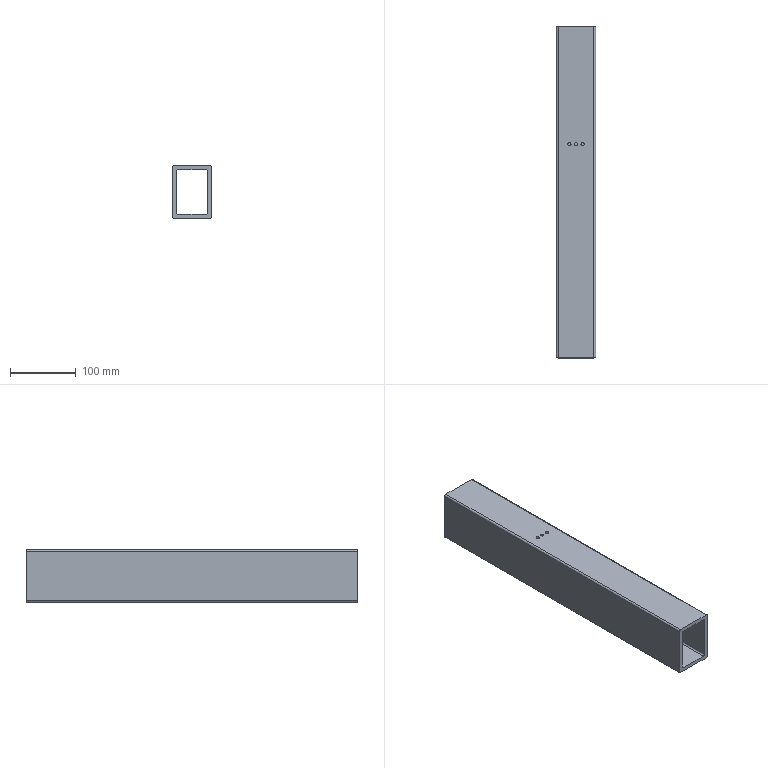Part | NX | 1 solid | 21 faces | box 60 x 505 x 80 mm | volume 775327 mm3 | cylinder 11 | plane 10 | commonest cylinder face diameters 5.236 x8 5 x3
STEP:
#1=CARTESIAN_POINT('',(746.,505.,37.382));
#2=VERTEX_POINT('',#1);
#3=CARTESIAN_POINT('',(746.,505.,-37.382));
#4=VERTEX_POINT('',#3);
#5=CARTESIAN_POINT('',(746.,505.,-37.382));
#6=DIRECTION('',(0.,0.,-1.));
#7=VECTOR('',#6,1000.);
#8=LINE('',#5,#7);
#9=EDGE_CURVE('',#2,#4,#8,.T.);
#10=ORIENTED_EDGE('',*,*,#9,.F.);
#11=CARTESIAN_POINT('',(746.,0.,37.382));
#12=VERTEX_POINT('',#11);
#13=CARTESIAN_POINT('',(746.,535.,37.382));
#14=DIRECTION('',(0.,-1.,0.));
#15=VECTOR('',#14,1000.);
#16=LINE('',#13,#15);
#17=EDGE_CURVE('',#2,#12,#16,.T.);
#18=ORIENTED_EDGE('',*,*,#17,.T.);
#19=CARTESIAN_POINT('',(746.,0.,-37.382));
#20=VERTEX_POINT('',#19);
#21=CARTESIAN_POINT('',(746.,0.,-37.382));
#22=DIRECTION('',(0.,0.,-1.));
#23=VECTOR('',#22,1000.);
#24=LINE('',#21,#23);
#25=EDGE_CURVE('',#12,#20,#24,.T.);
#26=ORIENTED_EDGE('',*,*,#25,.T.);
#27=CARTESIAN_POINT('',(746.,535.,-37.382));
#28=DIRECTION('',(0.,-1.,0.));
#29=VECTOR('',#28,1000.);
#30=LINE('',#27,#29);
#31=EDGE_CURVE('',#4,#20,#30,.T.);
#32=ORIENTED_EDGE('',*,*,#31,.F.);
#33=EDGE_LOOP('',(#10,#18,#26,#32));
#34=FACE_BOUND('',#33,.T.);
#35=CARTESIAN_POINT('',(746.,535.,-37.382));
#36=DIRECTION('',(-1.,0.,0.));
#37=DIRECTION('',(0.,0.,1.));
#38=AXIS2_PLACEMENT_3D('',#35,#36,#37);
#39=PLANE('',#38);
#40=ADVANCED_FACE('',(#34),#39,.F.);
#41=CARTESIAN_POINT('',(743.382,505.,40.));
#42=VERTEX_POINT('',#41);
#43=CARTESIAN_POINT('',(743.382,505.,37.382));
#44=DIRECTION('',(0.,1.,0.));
#45=DIRECTION('',(0.,0.,1.));
#46=AXIS2_PLACEMENT_3D('',#43,#44,#45);
#47=CIRCLE('',#46,2.618);
#48=EDGE_CURVE('',#42,#2,#47,.T.);
#49=ORIENTED_EDGE('',*,*,#48,.F.);
#50=CARTESIAN_POINT('',(743.382,0.,40.));
#51=VERTEX_POINT('',#50);
#52=CARTESIAN_POINT('',(743.382,535.,40.));
#53=DIRECTION('',(0.,-1.,0.));
#54=VECTOR('',#53,1000.);
#55=LINE('',#52,#54);
#56=EDGE_CURVE('',#42,#51,#55,.T.);
#57=ORIENTED_EDGE('',*,*,#56,.T.);
#58=CARTESIAN_POINT('',(743.382,0.,37.382));
#59=DIRECTION('',(0.,1.,0.));
#60=DIRECTION('',(0.,0.,1.));
#61=AXIS2_PLACEMENT_3D('',#58,#59,#60);
#62=CIRCLE('',#61,2.618);
#63=EDGE_CURVE('',#51,#12,#62,.T.);
#64=ORIENTED_EDGE('',*,*,#63,.T.);
#65=ORIENTED_EDGE('',*,*,#17,.F.);
#66=EDGE_LOOP('',(#49,#57,#64,#65));
#67=FACE_BOUND('',#66,.T.);
#68=CARTESIAN_POINT('',(743.382,535.,37.382));
#69=DIRECTION('',(0.,-1.,0.));
#70=DIRECTION('',(0.,0.,-1.));
#71=AXIS2_PLACEMENT_3D('',#68,#69,#70);
#72=CYLINDRICAL_SURFACE('',#71,2.618);
#73=ADVANCED_FACE('',(#67),#72,.T.);
#74=CARTESIAN_POINT('',(726.,322.5,40.));
#75=VERTEX_POINT('',#74);
#76=CARTESIAN_POINT('',(726.,325.,40.));
#77=DIRECTION('',(0.,0.,1.));
#78=DIRECTION('',(0.,-1.,0.));
#79=AXIS2_PLACEMENT_3D('',#76,#77,#78);
#80=CIRCLE('',#79,2.5);
#81=EDGE_CURVE('',#75,#75,#80,.T.);
#82=ORIENTED_EDGE('',*,*,#81,.F.);
#83=EDGE_LOOP('',(#82));
#84=FACE_BOUND('',#83,.T.);
#85=CARTESIAN_POINT('',(716.,322.5,40.));
#86=VERTEX_POINT('',#85);
#87=CARTESIAN_POINT('',(716.,325.,40.));
#88=DIRECTION('',(0.,0.,1.));
#89=DIRECTION('',(0.,-1.,0.));
#90=AXIS2_PLACEMENT_3D('',#87,#88,#89);
#91=CIRCLE('',#90,2.5);
#92=EDGE_CURVE('',#86,#86,#91,.T.);
#93=ORIENTED_EDGE('',*,*,#92,.F.);
#94=EDGE_LOOP('',(#93));
#95=FACE_BOUND('',#94,.T.);
#96=CARTESIAN_POINT('',(706.,322.5,40.));
#97=VERTEX_POINT('',#96);
#98=CARTESIAN_POINT('',(706.,325.,40.));
#99=DIRECTION('',(0.,0.,1.));
#100=DIRECTION('',(0.,-1.,0.));
#101=AXIS2_PLACEMENT_3D('',#98,#99,#100);
#102=CIRCLE('',#101,2.5);
#103=EDGE_CURVE('',#97,#97,#102,.T.);
#104=ORIENTED_EDGE('',*,*,#103,.F.);
#105=EDGE_LOOP('',(#104));
#106=FACE_BOUND('',#105,.T.);
#107=CARTESIAN_POINT('',(688.618,505.,40.));
#108=VERTEX_POINT('',#107);
#109=CARTESIAN_POINT('',(1126.,505.,40.));
#110=DIRECTION('',(-1.,0.,0.));
#111=VECTOR('',#110,1000.);
#112=LINE('',#109,#111);
#113=EDGE_CURVE('',#42,#108,#112,.T.);
#114=ORIENTED_EDGE('',*,*,#113,.T.);
#115=CARTESIAN_POINT('',(688.618,0.,40.));
#116=VERTEX_POINT('',#115);
#117=CARTESIAN_POINT('',(688.618,535.,40.));
#118=DIRECTION('',(0.,-1.,0.));
#119=VECTOR('',#118,1000.);
#120=LINE('',#117,#119);
#121=EDGE_CURVE('',#108,#116,#120,.T.);
#122=ORIENTED_EDGE('',*,*,#121,.T.);
#123=CARTESIAN_POINT('',(688.618,0.,40.));
#124=DIRECTION('',(1.,0.,0.));
#125=VECTOR('',#124,1000.);
#126=LINE('',#123,#125);
#127=EDGE_CURVE('',#116,#51,#126,.T.);
#128=ORIENTED_EDGE('',*,*,#127,.T.);
#129=ORIENTED_EDGE('',*,*,#56,.F.);
#130=EDGE_LOOP('',(#114,#122,#128,#129));
#131=FACE_BOUND('',#130,.T.);
#132=CARTESIAN_POINT('',(688.618,535.,40.));
#133=DIRECTION('',(0.,0.,-1.));
#134=DIRECTION('',(-1.,0.,0.));
#135=AXIS2_PLACEMENT_3D('',#132,#133,#134);
#136=PLANE('',#135);
#137=ADVANCED_FACE('',(#84,#95,#106,#131),#136,.F.);
#138=CARTESIAN_POINT('',(686.,505.,37.382));
#139=VERTEX_POINT('',#138);
#140=CARTESIAN_POINT('',(688.618,505.,37.382));
#141=DIRECTION('',(0.,1.,0.));
#142=DIRECTION('',(0.,0.,1.));
#143=AXIS2_PLACEMENT_3D('',#140,#141,#142);
#144=CIRCLE('',#143,2.618);
#145=EDGE_CURVE('',#139,#108,#144,.T.);
#146=ORIENTED_EDGE('',*,*,#145,.F.);
#147=CARTESIAN_POINT('',(686.,0.,37.382));
#148=VERTEX_POINT('',#147);
#149=CARTESIAN_POINT('',(686.,535.,37.382));
#150=DIRECTION('',(0.,-1.,0.));
#151=VECTOR('',#150,1000.);
#152=LINE('',#149,#151);
#153=EDGE_CURVE('',#139,#148,#152,.T.);
#154=ORIENTED_EDGE('',*,*,#153,.T.);
#155=CARTESIAN_POINT('',(688.618,0.,37.382));
#156=DIRECTION('',(0.,1.,0.));
#157=DIRECTION('',(0.,0.,1.));
#158=AXIS2_PLACEMENT_3D('',#155,#156,#157);
#159=CIRCLE('',#158,2.618);
#160=EDGE_CURVE('',#148,#116,#159,.T.);
#161=ORIENTED_EDGE('',*,*,#160,.T.);
#162=ORIENTED_EDGE('',*,*,#121,.F.);
#163=EDGE_LOOP('',(#146,#154,#161,#162));
#164=FACE_BOUND('',#163,.T.);
#165=CARTESIAN_POINT('',(688.618,535.,37.382));
#166=DIRECTION('',(0.,-1.,0.));
#167=DIRECTION('',(0.,0.,-1.));
#168=AXIS2_PLACEMENT_3D('',#165,#166,#167);
#169=CYLINDRICAL_SURFACE('',#168,2.618);
#170=ADVANCED_FACE('',(#164),#169,.T.);
#171=CARTESIAN_POINT('',(686.,505.,-37.382));
#172=VERTEX_POINT('',#171);
#173=CARTESIAN_POINT('',(686.,505.,-37.382));
#174=DIRECTION('',(0.,0.,1.));
#175=VECTOR('',#174,1000.);
#176=LINE('',#173,#175);
#177=EDGE_CURVE('',#172,#139,#176,.T.);
#178=ORIENTED_EDGE('',*,*,#177,.F.);
#179=CARTESIAN_POINT('',(686.,0.,-37.382));
#180=VERTEX_POINT('',#179);
#181=CARTESIAN_POINT('',(686.,535.,-37.382));
#182=DIRECTION('',(0.,-1.,0.));
#183=VECTOR('',#182,1000.);
#184=LINE('',#181,#183);
#185=EDGE_CURVE('',#172,#180,#184,.T.);
#186=ORIENTED_EDGE('',*,*,#185,.T.);
#187=CARTESIAN_POINT('',(686.,0.,-37.382));
#188=DIRECTION('',(0.,0.,1.));
#189=VECTOR('',#188,1000.);
#190=LINE('',#187,#189);
#191=EDGE_CURVE('',#180,#148,#190,.T.);
#192=ORIENTED_EDGE('',*,*,#191,.T.);
#193=ORIENTED_EDGE('',*,*,#153,.F.);
#194=EDGE_LOOP('',(#178,#186,#192,#193));
#195=FACE_BOUND('',#194,.T.);
#196=CARTESIAN_POINT('',(686.,535.,-37.382));
#197=DIRECTION('',(1.,0.,0.));
#198=DIRECTION('',(0.,0.,-1.));
#199=AXIS2_PLACEMENT_3D('',#196,#197,#198);
#200=PLANE('',#199);
#201=ADVANCED_FACE('',(#195),#200,.F.);
#202=CARTESIAN_POINT('',(688.618,505.,-40.));
#203=VERTEX_POINT('',#202);
#204=CARTESIAN_POINT('',(688.618,505.,-37.382));
#205=DIRECTION('',(0.,1.,0.));
#206=DIRECTION('',(0.,0.,1.));
#207=AXIS2_PLACEMENT_3D('',#204,#205,#206);
#208=CIRCLE('',#207,2.618);
#209=EDGE_CURVE('',#203,#172,#208,.T.);
#210=ORIENTED_EDGE('',*,*,#209,.F.);
#211=CARTESIAN_POINT('',(688.618,0.,-40.));
#212=VERTEX_POINT('',#211);
#213=CARTESIAN_POINT('',(688.618,535.,-40.));
#214=DIRECTION('',(0.,-1.,0.));
#215=VECTOR('',#214,1000.);
#216=LINE('',#213,#215);
#217=EDGE_CURVE('',#203,#212,#216,.T.);
#218=ORIENTED_EDGE('',*,*,#217,.T.);
#219=CARTESIAN_POINT('',(688.618,0.,-37.382));
#220=DIRECTION('',(0.,1.,0.));
#221=DIRECTION('',(0.,0.,1.));
#222=AXIS2_PLACEMENT_3D('',#219,#220,#221);
#223=CIRCLE('',#222,2.618);
#224=EDGE_CURVE('',#212,#180,#223,.T.);
#225=ORIENTED_EDGE('',*,*,#224,.T.);
#226=ORIENTED_EDGE('',*,*,#185,.F.);
#227=EDGE_LOOP('',(#210,#218,#225,#226));
#228=FACE_BOUND('',#227,.T.);
#229=CARTESIAN_POINT('',(688.618,535.,-37.382));
#230=DIRECTION('',(0.,-1.,0.));
#231=DIRECTION('',(0.,0.,-1.));
#232=AXIS2_PLACEMENT_3D('',#229,#230,#231);
#233=CYLINDRICAL_SURFACE('',#232,2.618);
#234=ADVANCED_FACE('',(#228),#233,.T.);
#235=CARTESIAN_POINT('',(743.382,505.,-40.));
#236=VERTEX_POINT('',#235);
#237=CARTESIAN_POINT('',(1126.,505.,-40.));
#238=DIRECTION('',(-1.,0.,0.));
#239=VECTOR('',#238,1000.);
#240=LINE('',#237,#239);
#241=EDGE_CURVE('',#236,#203,#240,.T.);
#242=ORIENTED_EDGE('',*,*,#241,.F.);
#243=CARTESIAN_POINT('',(743.382,0.,-40.));
#244=VERTEX_POINT('',#243);
#245=CARTESIAN_POINT('',(743.382,535.,-40.));
#246=DIRECTION('',(0.,-1.,0.));
#247=VECTOR('',#246,1000.);
#248=LINE('',#245,#247);
#249=EDGE_CURVE('',#236,#244,#248,.T.);
#250=ORIENTED_EDGE('',*,*,#249,.T.);
#251=CARTESIAN_POINT('',(688.618,0.,-40.));
#252=DIRECTION('',(-1.,0.,0.));
#253=VECTOR('',#252,1000.);
#254=LINE('',#251,#253);
#255=EDGE_CURVE('',#244,#212,#254,.T.);
#256=ORIENTED_EDGE('',*,*,#255,.T.);
#257=ORIENTED_EDGE('',*,*,#217,.F.);
#258=EDGE_LOOP('',(#242,#250,#256,#257));
#259=FACE_BOUND('',#258,.T.);
#260=CARTESIAN_POINT('',(688.618,535.,-40.));
#261=DIRECTION('',(0.,0.,1.));
#262=DIRECTION('',(1.,0.,0.));
#263=AXIS2_PLACEMENT_3D('',#260,#261,#262);
#264=PLANE('',#263);
#265=ADVANCED_FACE('',(#259),#264,.F.);
#266=CARTESIAN_POINT('',(743.382,505.,-37.382));
#267=DIRECTION('',(0.,1.,0.));
#268=DIRECTION('',(0.,0.,1.));
#269=AXIS2_PLACEMENT_3D('',#266,#267,#268);
#270=CIRCLE('',#269,2.618);
#271=EDGE_CURVE('',#4,#236,#270,.T.);
#272=ORIENTED_EDGE('',*,*,#271,.F.);
#273=ORIENTED_EDGE('',*,*,#31,.T.);
#274=CARTESIAN_POINT('',(743.382,0.,-37.382));
#275=DIRECTION('',(0.,1.,0.));
#276=DIRECTION('',(0.,0.,-1.));
#277=AXIS2_PLACEMENT_3D('',#274,#275,#276);
#278=CIRCLE('',#277,2.618);
#279=EDGE_CURVE('',#20,#244,#278,.T.);
#280=ORIENTED_EDGE('',*,*,#279,.T.);
#281=ORIENTED_EDGE('',*,*,#249,.F.);
#282=EDGE_LOOP('',(#272,#273,#280,#281));
#283=FACE_BOUND('',#282,.T.);
#284=CARTESIAN_POINT('',(743.382,535.,-37.382));
#285=DIRECTION('',(0.,-1.,0.));
#286=DIRECTION('',(0.,0.,-1.));
#287=AXIS2_PLACEMENT_3D('',#284,#285,#286);
#288=CYLINDRICAL_SURFACE('',#287,2.618);
#289=ADVANCED_FACE('',(#283),#288,.T.);
#290=ORIENTED_EDGE('',*,*,#279,.F.);
#291=ORIENTED_EDGE('',*,*,#25,.F.);
#292=ORIENTED_EDGE('',*,*,#63,.F.);
#293=ORIENTED_EDGE('',*,*,#127,.F.);
#294=ORIENTED_EDGE('',*,*,#160,.F.);
#295=ORIENTED_EDGE('',*,*,#191,.F.);
#296=ORIENTED_EDGE('',*,*,#224,.F.);
#297=ORIENTED_EDGE('',*,*,#255,.F.);
#298=EDGE_LOOP('',(#290,#291,#292,#293,#294,#295,#296,#297));
#299=FACE_BOUND('',#298,.T.);
#300=CARTESIAN_POINT('',(692.,0.,31.382));
#301=VERTEX_POINT('',#300);
#302=CARTESIAN_POINT('',(694.618,0.,34.));
#303=VERTEX_POINT('',#302);
#304=CARTESIAN_POINT('',(694.618,0.,31.382));
#305=DIRECTION('',(0.,1.,0.));
#306=DIRECTION('',(0.,0.,-1.));
#307=AXIS2_PLACEMENT_3D('',#304,#305,#306);
#308=CIRCLE('',#307,2.618);
#309=EDGE_CURVE('',#301,#303,#308,.T.);
#310=ORIENTED_EDGE('',*,*,#309,.T.);
#311=CARTESIAN_POINT('',(737.382,0.,34.));
#312=VERTEX_POINT('',#311);
#313=CARTESIAN_POINT('',(694.618,0.,34.));
#314=DIRECTION('',(1.,0.,0.));
#315=VECTOR('',#314,1000.);
#316=LINE('',#313,#315);
#317=EDGE_CURVE('',#303,#312,#316,.T.);
#318=ORIENTED_EDGE('',*,*,#317,.T.);
#319=CARTESIAN_POINT('',(740.,0.,31.382));
#320=VERTEX_POINT('',#319);
#321=CARTESIAN_POINT('',(737.382,0.,31.382));
#322=DIRECTION('',(0.,1.,0.));
#323=DIRECTION('',(0.,0.,-1.));
#324=AXIS2_PLACEMENT_3D('',#321,#322,#323);
#325=CIRCLE('',#324,2.618);
#326=EDGE_CURVE('',#312,#320,#325,.T.);
#327=ORIENTED_EDGE('',*,*,#326,.T.);
#328=CARTESIAN_POINT('',(740.,0.,-31.382));
#329=VERTEX_POINT('',#328);
#330=CARTESIAN_POINT('',(740.,0.,-31.382));
#331=DIRECTION('',(0.,0.,-1.));
#332=VECTOR('',#331,1000.);
#333=LINE('',#330,#332);
#334=EDGE_CURVE('',#320,#329,#333,.T.);
#335=ORIENTED_EDGE('',*,*,#334,.T.);
#336=CARTESIAN_POINT('',(737.382,0.,-34.));
#337=VERTEX_POINT('',#336);
#338=CARTESIAN_POINT('',(737.382,0.,-31.382));
#339=DIRECTION('',(0.,1.,0.));
#340=DIRECTION('',(0.,0.,-1.));
#341=AXIS2_PLACEMENT_3D('',#338,#339,#340);
#342=CIRCLE('',#341,2.618);
#343=EDGE_CURVE('',#329,#337,#342,.T.);
#344=ORIENTED_EDGE('',*,*,#343,.T.);
#345=CARTESIAN_POINT('',(694.618,0.,-34.));
#346=VERTEX_POINT('',#345);
#347=CARTESIAN_POINT('',(694.618,0.,-34.));
#348=DIRECTION('',(-1.,0.,0.));
#349=VECTOR('',#348,1000.);
#350=LINE('',#347,#349);
#351=EDGE_CURVE('',#337,#346,#350,.T.);
#352=ORIENTED_EDGE('',*,*,#351,.T.);
#353=CARTESIAN_POINT('',(692.,0.,-31.382));
#354=VERTEX_POINT('',#353);
#355=CARTESIAN_POINT('',(694.618,0.,-31.382));
#356=DIRECTION('',(0.,1.,0.));
#357=DIRECTION('',(0.,0.,1.));
#358=AXIS2_PLACEMENT_3D('',#355,#356,#357);
#359=CIRCLE('',#358,2.618);
#360=EDGE_CURVE('',#346,#354,#359,.T.);
#361=ORIENTED_EDGE('',*,*,#360,.T.);
#362=CARTESIAN_POINT('',(692.,0.,-31.382));
#363=DIRECTION('',(0.,0.,1.));
#364=VECTOR('',#363,1000.);
#365=LINE('',#362,#364);
#366=EDGE_CURVE('',#354,#301,#365,.T.);
#367=ORIENTED_EDGE('',*,*,#366,.T.);
#368=EDGE_LOOP('',(#310,#318,#327,#335,#344,#352,#361,#367));
#369=FACE_BOUND('',#368,.T.);
#370=CARTESIAN_POINT('',(743.382,0.,-37.382));
#371=DIRECTION('',(0.,-1.,0.));
#372=DIRECTION('',(0.,0.,-1.));
#373=AXIS2_PLACEMENT_3D('',#370,#371,#372);
#374=PLANE('',#373);
#375=ADVANCED_FACE('',(#299,#369),#374,.T.);
#376=CARTESIAN_POINT('',(723.5,325.,34.));
#377=VERTEX_POINT('',#376);
#378=CARTESIAN_POINT('',(726.,325.,34.));
#379=DIRECTION('',(0.,0.,-1.));
#380=DIRECTION('',(-1.,0.,0.));
#381=AXIS2_PLACEMENT_3D('',#378,#379,#380);
#382=CIRCLE('',#381,2.5);
#383=EDGE_CURVE('',#377,#377,#382,.T.);
#384=ORIENTED_EDGE('',*,*,#383,.F.);
#385=EDGE_LOOP('',(#384));
#386=FACE_BOUND('',#385,.T.);
#387=CARTESIAN_POINT('',(713.5,325.,34.));
#388=VERTEX_POINT('',#387);
#389=CARTESIAN_POINT('',(716.,325.,34.));
#390=DIRECTION('',(0.,0.,-1.));
#391=DIRECTION('',(-1.,0.,0.));
#392=AXIS2_PLACEMENT_3D('',#389,#390,#391);
#393=CIRCLE('',#392,2.5);
#394=EDGE_CURVE('',#388,#388,#393,.T.);
#395=ORIENTED_EDGE('',*,*,#394,.F.);
#396=EDGE_LOOP('',(#395));
#397=FACE_BOUND('',#396,.T.);
#398=CARTESIAN_POINT('',(703.5,325.,34.));
#399=VERTEX_POINT('',#398);
#400=CARTESIAN_POINT('',(706.,325.,34.));
#401=DIRECTION('',(0.,0.,-1.));
#402=DIRECTION('',(-1.,0.,0.));
#403=AXIS2_PLACEMENT_3D('',#400,#401,#402);
#404=CIRCLE('',#403,2.5);
#405=EDGE_CURVE('',#399,#399,#404,.T.);
#406=ORIENTED_EDGE('',*,*,#405,.F.);
#407=EDGE_LOOP('',(#406));
#408=FACE_BOUND('',#407,.T.);
#409=CARTESIAN_POINT('',(694.618,505.,34.));
#410=VERTEX_POINT('',#409);
#411=CARTESIAN_POINT('',(694.618,535.,34.));
#412=DIRECTION('',(0.,-1.,0.));
#413=VECTOR('',#412,1000.);
#414=LINE('',#411,#413);
#415=EDGE_CURVE('',#410,#303,#414,.T.);
#416=ORIENTED_EDGE('',*,*,#415,.F.);
#417=CARTESIAN_POINT('',(737.382,505.,34.));
#418=VERTEX_POINT('',#417);
#419=CARTESIAN_POINT('',(694.618,505.,34.));
#420=DIRECTION('',(1.,0.,0.));
#421=VECTOR('',#420,1000.);
#422=LINE('',#419,#421);
#423=EDGE_CURVE('',#410,#418,#422,.T.);
#424=ORIENTED_EDGE('',*,*,#423,.T.);
#425=CARTESIAN_POINT('',(737.382,535.,34.));
#426=DIRECTION('',(0.,-1.,0.));
#427=VECTOR('',#426,1000.);
#428=LINE('',#425,#427);
#429=EDGE_CURVE('',#418,#312,#428,.T.);
#430=ORIENTED_EDGE('',*,*,#429,.T.);
#431=ORIENTED_EDGE('',*,*,#317,.F.);
#432=EDGE_LOOP('',(#416,#424,#430,#431));
#433=FACE_BOUND('',#432,.T.);
#434=CARTESIAN_POINT('',(694.618,535.,34.));
#435=DIRECTION('',(0.,0.,-1.));
#436=DIRECTION('',(-1.,0.,0.));
#437=AXIS2_PLACEMENT_3D('',#434,#435,#436);
#438=PLANE('',#437);
#439=ADVANCED_FACE('',(#386,#397,#408,#433),#438,.T.);
#440=ORIENTED_EDGE('',*,*,#429,.F.);
#441=CARTESIAN_POINT('',(740.,505.,31.382));
#442=VERTEX_POINT('',#441);
#443=CARTESIAN_POINT('',(737.382,505.,31.382));
#444=DIRECTION('',(0.,1.,0.));
#445=DIRECTION('',(0.,0.,1.));
#446=AXIS2_PLACEMENT_3D('',#443,#444,#445);
#447=CIRCLE('',#446,2.618);
#448=EDGE_CURVE('',#418,#442,#447,.T.);
#449=ORIENTED_EDGE('',*,*,#448,.T.);
#450=CARTESIAN_POINT('',(740.,535.,31.382));
#451=DIRECTION('',(0.,-1.,0.));
#452=VECTOR('',#451,1000.);
#453=LINE('',#450,#452);
#454=EDGE_CURVE('',#442,#320,#453,.T.);
#455=ORIENTED_EDGE('',*,*,#454,.T.);
#456=ORIENTED_EDGE('',*,*,#326,.F.);
#457=EDGE_LOOP('',(#440,#449,#455,#456));
#458=FACE_BOUND('',#457,.T.);
#459=CARTESIAN_POINT('',(737.382,535.,31.382));
#460=DIRECTION('',(0.,-1.,0.));
#461=DIRECTION('',(0.,0.,-1.));
#462=AXIS2_PLACEMENT_3D('',#459,#460,#461);
#463=CYLINDRICAL_SURFACE('',#462,2.618);
#464=ADVANCED_FACE('',(#458),#463,.F.);
#465=ORIENTED_EDGE('',*,*,#454,.F.);
#466=CARTESIAN_POINT('',(740.,505.,-31.382));
#467=VERTEX_POINT('',#466);
#468=CARTESIAN_POINT('',(740.,505.,-31.382));
#469=DIRECTION('',(0.,0.,-1.));
#470=VECTOR('',#469,1000.);
#471=LINE('',#468,#470);
#472=EDGE_CURVE('',#442,#467,#471,.T.);
#473=ORIENTED_EDGE('',*,*,#472,.T.);
#474=CARTESIAN_POINT('',(740.,535.,-31.382));
#475=DIRECTION('',(0.,-1.,0.));
#476=VECTOR('',#475,1000.);
#477=LINE('',#474,#476);
#478=EDGE_CURVE('',#467,#329,#477,.T.);
#479=ORIENTED_EDGE('',*,*,#478,.T.);
#480=ORIENTED_EDGE('',*,*,#334,.F.);
#481=EDGE_LOOP('',(#465,#473,#479,#480));
#482=FACE_BOUND('',#481,.T.);
#483=CARTESIAN_POINT('',(740.,535.,-31.382));
#484=DIRECTION('',(-1.,0.,0.));
#485=DIRECTION('',(0.,0.,1.));
#486=AXIS2_PLACEMENT_3D('',#483,#484,#485);
#487=PLANE('',#486);
#488=ADVANCED_FACE('',(#482),#487,.T.);
#489=ORIENTED_EDGE('',*,*,#478,.F.);
#490=CARTESIAN_POINT('',(737.382,505.,-34.));
#491=VERTEX_POINT('',#490);
#492=CARTESIAN_POINT('',(737.382,505.,-31.382));
#493=DIRECTION('',(0.,1.,0.));
#494=DIRECTION('',(0.,0.,1.));
#495=AXIS2_PLACEMENT_3D('',#492,#493,#494);
#496=CIRCLE('',#495,2.618);
#497=EDGE_CURVE('',#467,#491,#496,.T.);
#498=ORIENTED_EDGE('',*,*,#497,.T.);
#499=CARTESIAN_POINT('',(737.382,535.,-34.));
#500=DIRECTION('',(0.,-1.,0.));
#501=VECTOR('',#500,1000.);
#502=LINE('',#499,#501);
#503=EDGE_CURVE('',#491,#337,#502,.T.);
#504=ORIENTED_EDGE('',*,*,#503,.T.);
#505=ORIENTED_EDGE('',*,*,#343,.F.);
#506=EDGE_LOOP('',(#489,#498,#504,#505));
#507=FACE_BOUND('',#506,.T.);
#508=CARTESIAN_POINT('',(737.382,535.,-31.382));
#509=DIRECTION('',(0.,-1.,0.));
#510=DIRECTION('',(0.,0.,-1.));
#511=AXIS2_PLACEMENT_3D('',#508,#509,#510);
#512=CYLINDRICAL_SURFACE('',#511,2.618);
#513=ADVANCED_FACE('',(#507),#512,.F.);
#514=ORIENTED_EDGE('',*,*,#503,.F.);
#515=CARTESIAN_POINT('',(694.618,505.,-34.));
#516=VERTEX_POINT('',#515);
#517=CARTESIAN_POINT('',(694.618,505.,-34.));
#518=DIRECTION('',(-1.,0.,0.));
#519=VECTOR('',#518,1000.);
#520=LINE('',#517,#519);
#521=EDGE_CURVE('',#491,#516,#520,.T.);
#522=ORIENTED_EDGE('',*,*,#521,.T.);
#523=CARTESIAN_POINT('',(694.618,535.,-34.));
#524=DIRECTION('',(0.,-1.,0.));
#525=VECTOR('',#524,1000.);
#526=LINE('',#523,#525);
#527=EDGE_CURVE('',#516,#346,#526,.T.);
#528=ORIENTED_EDGE('',*,*,#527,.T.);
#529=ORIENTED_EDGE('',*,*,#351,.F.);
#530=EDGE_LOOP('',(#514,#522,#528,#529));
#531=FACE_BOUND('',#530,.T.);
#532=CARTESIAN_POINT('',(694.618,535.,-34.));
#533=DIRECTION('',(0.,0.,1.));
#534=DIRECTION('',(1.,0.,0.));
#535=AXIS2_PLACEMENT_3D('',#532,#533,#534);
#536=PLANE('',#535);
#537=ADVANCED_FACE('',(#531),#536,.T.);
#538=ORIENTED_EDGE('',*,*,#527,.F.);
#539=CARTESIAN_POINT('',(692.,505.,-31.382));
#540=VERTEX_POINT('',#539);
#541=CARTESIAN_POINT('',(694.618,505.,-31.382));
#542=DIRECTION('',(0.,1.,0.));
#543=DIRECTION('',(0.,0.,1.));
#544=AXIS2_PLACEMENT_3D('',#541,#542,#543);
#545=CIRCLE('',#544,2.618);
#546=EDGE_CURVE('',#516,#540,#545,.T.);
#547=ORIENTED_EDGE('',*,*,#546,.T.);
#548=CARTESIAN_POINT('',(692.,535.,-31.382));
#549=DIRECTION('',(0.,-1.,0.));
#550=VECTOR('',#549,1000.);
#551=LINE('',#548,#550);
#552=EDGE_CURVE('',#540,#354,#551,.T.);
#553=ORIENTED_EDGE('',*,*,#552,.T.);
#554=ORIENTED_EDGE('',*,*,#360,.F.);
#555=EDGE_LOOP('',(#538,#547,#553,#554));
#556=FACE_BOUND('',#555,.T.);
#557=CARTESIAN_POINT('',(694.618,535.,-31.382));
#558=DIRECTION('',(0.,-1.,0.));
#559=DIRECTION('',(0.,0.,-1.));
#560=AXIS2_PLACEMENT_3D('',#557,#558,#559);
#561=CYLINDRICAL_SURFACE('',#560,2.618);
#562=ADVANCED_FACE('',(#556),#561,.F.);
#563=ORIENTED_EDGE('',*,*,#552,.F.);
#564=CARTESIAN_POINT('',(692.,505.,31.382));
#565=VERTEX_POINT('',#564);
#566=CARTESIAN_POINT('',(692.,505.,-31.382));
#567=DIRECTION('',(0.,0.,1.));
#568=VECTOR('',#567,1000.);
#569=LINE('',#566,#568);
#570=EDGE_CURVE('',#540,#565,#569,.T.);
#571=ORIENTED_EDGE('',*,*,#570,.T.);
#572=CARTESIAN_POINT('',(692.,535.,31.382));
#573=DIRECTION('',(0.,-1.,0.));
#574=VECTOR('',#573,1000.);
#575=LINE('',#572,#574);
#576=EDGE_CURVE('',#565,#301,#575,.T.);
#577=ORIENTED_EDGE('',*,*,#576,.T.);
#578=ORIENTED_EDGE('',*,*,#366,.F.);
#579=EDGE_LOOP('',(#563,#571,#577,#578));
#580=FACE_BOUND('',#579,.T.);
#581=CARTESIAN_POINT('',(692.,535.,-31.382));
#582=DIRECTION('',(1.,0.,0.));
#583=DIRECTION('',(0.,0.,-1.));
#584=AXIS2_PLACEMENT_3D('',#581,#582,#583);
#585=PLANE('',#584);
#586=ADVANCED_FACE('',(#580),#585,.T.);
#587=ORIENTED_EDGE('',*,*,#576,.F.);
#588=CARTESIAN_POINT('',(694.618,505.,31.382));
#589=DIRECTION('',(0.,1.,0.));
#590=DIRECTION('',(0.,0.,1.));
#591=AXIS2_PLACEMENT_3D('',#588,#589,#590);
#592=CIRCLE('',#591,2.618);
#593=EDGE_CURVE('',#565,#410,#592,.T.);
#594=ORIENTED_EDGE('',*,*,#593,.T.);
#595=ORIENTED_EDGE('',*,*,#415,.T.);
#596=ORIENTED_EDGE('',*,*,#309,.F.);
#597=EDGE_LOOP('',(#587,#594,#595,#596));
#598=FACE_BOUND('',#597,.T.);
#599=CARTESIAN_POINT('',(694.618,535.,31.382));
#600=DIRECTION('',(0.,-1.,0.));
#601=DIRECTION('',(0.,0.,-1.));
#602=AXIS2_PLACEMENT_3D('',#599,#600,#601);
#603=CYLINDRICAL_SURFACE('',#602,2.618);
#604=ADVANCED_FACE('',(#598),#603,.F.);
#605=ORIENTED_EDGE('',*,*,#570,.F.);
#606=ORIENTED_EDGE('',*,*,#546,.F.);
#607=ORIENTED_EDGE('',*,*,#521,.F.);
#608=ORIENTED_EDGE('',*,*,#497,.F.);
#609=ORIENTED_EDGE('',*,*,#472,.F.);
#610=ORIENTED_EDGE('',*,*,#448,.F.);
#611=ORIENTED_EDGE('',*,*,#423,.F.);
#612=ORIENTED_EDGE('',*,*,#593,.F.);
#613=EDGE_LOOP('',(#605,#606,#607,#608,#609,#610,#611,#612));
#614=FACE_BOUND('',#613,.T.);
#615=ORIENTED_EDGE('',*,*,#209,.T.);
#616=ORIENTED_EDGE('',*,*,#177,.T.);
#617=ORIENTED_EDGE('',*,*,#145,.T.);
#618=ORIENTED_EDGE('',*,*,#113,.F.);
#619=ORIENTED_EDGE('',*,*,#48,.T.);
#620=ORIENTED_EDGE('',*,*,#9,.T.);
#621=ORIENTED_EDGE('',*,*,#271,.T.);
#622=ORIENTED_EDGE('',*,*,#241,.T.);
#623=EDGE_LOOP('',(#615,#616,#617,#618,#619,#620,#621,#622));
#624=FACE_BOUND('',#623,.T.);
#625=CARTESIAN_POINT('',(1126.,505.,37.382));
#626=DIRECTION('',(0.,1.,0.));
#627=DIRECTION('',(0.,0.,1.));
#628=AXIS2_PLACEMENT_3D('',#625,#626,#627);
#629=PLANE('',#628);
#630=ADVANCED_FACE('',(#614,#624),#629,.T.);
#631=ORIENTED_EDGE('',*,*,#405,.T.);
#632=EDGE_LOOP('',(#631));
#633=FACE_BOUND('',#632,.T.);
#634=ORIENTED_EDGE('',*,*,#103,.T.);
#635=EDGE_LOOP('',(#634));
#636=FACE_BOUND('',#635,.T.);
#637=CARTESIAN_POINT('',(706.,325.,40.));
#638=DIRECTION('',(0.,0.,1.));
#639=DIRECTION('',(0.,-1.,0.));
#640=AXIS2_PLACEMENT_3D('',#637,#638,#639);
#641=CYLINDRICAL_SURFACE('',#640,2.5);
#642=ADVANCED_FACE('',(#633,#636),#641,.F.);
#643=ORIENTED_EDGE('',*,*,#394,.T.);
#644=EDGE_LOOP('',(#643));
#645=FACE_BOUND('',#644,.T.);
#646=ORIENTED_EDGE('',*,*,#92,.T.);
#647=EDGE_LOOP('',(#646));
#648=FACE_BOUND('',#647,.T.);
#649=CARTESIAN_POINT('',(716.,325.,40.));
#650=DIRECTION('',(0.,0.,1.));
#651=DIRECTION('',(0.,-1.,0.));
#652=AXIS2_PLACEMENT_3D('',#649,#650,#651);
#653=CYLINDRICAL_SURFACE('',#652,2.5);
#654=ADVANCED_FACE('',(#645,#648),#653,.F.);
#655=ORIENTED_EDGE('',*,*,#383,.T.);
#656=EDGE_LOOP('',(#655));
#657=FACE_BOUND('',#656,.T.);
#658=ORIENTED_EDGE('',*,*,#81,.T.);
#659=EDGE_LOOP('',(#658));
#660=FACE_BOUND('',#659,.T.);
#661=CARTESIAN_POINT('',(726.,325.,40.));
#662=DIRECTION('',(0.,0.,1.));
#663=DIRECTION('',(0.,-1.,0.));
#664=AXIS2_PLACEMENT_3D('',#661,#662,#663);
#665=CYLINDRICAL_SURFACE('',#664,2.5);
#666=ADVANCED_FACE('',(#657,#660),#665,.F.);
#667=CLOSED_SHELL('',(#40,#73,#137,#170,#201,#234,#265,#289,#375,#439,#464,#488,#513,#537,#562,#586,#604,#630,#642,#654,#666));
#668=MANIFOLD_SOLID_BREP('',#667);
#669=(LENGTH_UNIT()NAMED_UNIT(*)SI_UNIT(.MILLI.,.METRE.));
#670=UNCERTAINTY_MEASURE_WITH_UNIT(LENGTH_MEASURE(0.00001),#669,'','');
#671=(NAMED_UNIT(*)PLANE_ANGLE_UNIT()SI_UNIT($,.RADIAN.));
#672=(NAMED_UNIT(*)SI_UNIT($,.STERADIAN.)SOLID_ANGLE_UNIT());
#673=(GEOMETRIC_REPRESENTATION_CONTEXT(3)GLOBAL_UNCERTAINTY_ASSIGNED_CONTEXT((#670))GLOBAL_UNIT_ASSIGNED_CONTEXT((#669,#671,#672))REPRESENTATION_CONTEXT('',''));
#674=ADVANCED_BREP_SHAPE_REPRESENTATION('',(#668),#673);